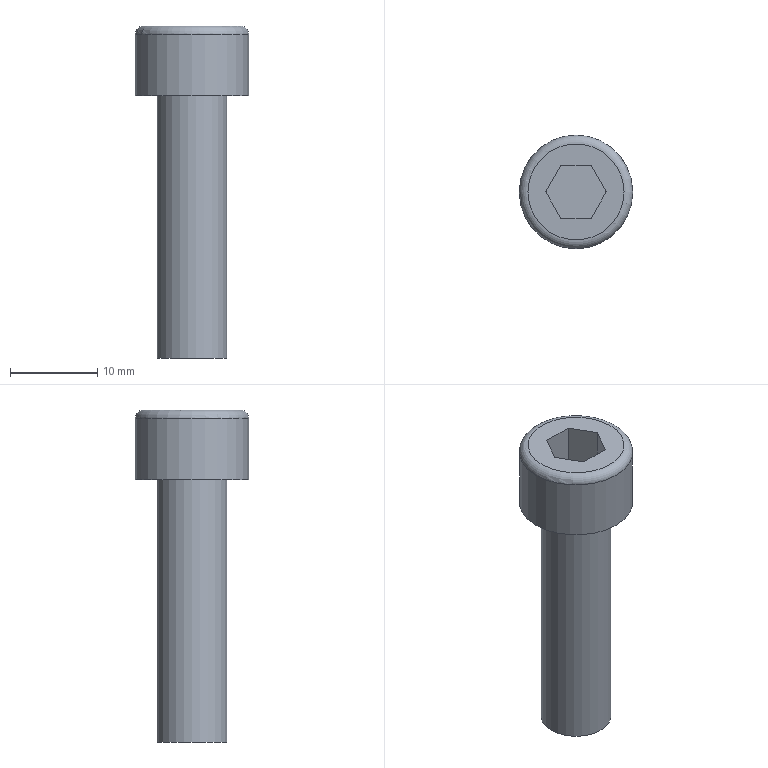Part | STEP file | Tube necking machine_id386_x_t | 1 solid | 13 faces | box 13 x 13 x 38 mm | volume 2397 mm3 | plane 10 | cylinder 2 | torus 1 | commonest cylinder face diameters 8 x1 13 x1
STEP:
#1=CARTESIAN_POINT('',(0.,0.,0.));
#2=DIRECTION('',(0.,0.,1.));
#3=DIRECTION('',(1.,0.,0.));
#4=AXIS2_PLACEMENT_3D('',#1,#2,#3);
#5=CARTESIAN_POINT('',(-164.,28.,208.));
#6=VERTEX_POINT('',#5);
#7=CARTESIAN_POINT('',(-169.5,28.,208.));
#8=DIRECTION('',(0.,0.,1.));
#9=DIRECTION('',(1.,0.,0.));
#10=AXIS2_PLACEMENT_3D('',#7,#8,#9);
#11=CIRCLE('',#10,5.5);
#12=CARTESIAN_POINT('',(-176.,28.,208.));
#13=DIRECTION('',(0.,0.,-1.));
#14=DIRECTION('',(1.,0.,0.));
#15=AXIS2_PLACEMENT_3D('',#12,#13,#14);
#16=PLANE('',#15);
#17=CARTESIAN_POINT('',(12.,0.));
#18=CARTESIAN_POINT('',(12.,-9.526));
#19=CARTESIAN_POINT('',(3.75,-4.763));
#20=CARTESIAN_POINT('',(-4.5,0.));
#21=CARTESIAN_POINT('',(3.75,4.763));
#22=CARTESIAN_POINT('',(12.,9.526));
#23=CARTESIAN_POINT('',(12.,0.));
#24=(BOUNDED_CURVE()B_SPLINE_CURVE(2,(#17,#18,#19,#20,#21,#22,#23),.UNSPECIFIED.,.T.,.F.)B_SPLINE_CURVE_WITH_KNOTS((1,2,2,2,2,1),(-2.094,0.,2.094,4.189,6.283,8.378),.UNSPECIFIED.)CURVE()GEOMETRIC_REPRESENTATION_ITEM()RATIONAL_B_SPLINE_CURVE((1.,0.5,1.,0.5,1.,0.5,1.))REPRESENTATION_ITEM(''));
#25=(GEOMETRIC_REPRESENTATION_CONTEXT(2)PARAMETRIC_REPRESENTATION_CONTEXT()REPRESENTATION_CONTEXT('',''));
#26=DEFINITIONAL_REPRESENTATION('',(#24),#25);
#27=PCURVE('',#16,#26);
#28=CARTESIAN_POINT('',(-169.5,28.,207.));
#29=DIRECTION('',(0.,0.,-1.));
#30=DIRECTION('',(1.,0.,0.));
#31=AXIS2_PLACEMENT_3D('',#28,#29,#30);
#32=TOROIDAL_SURFACE('',#31,5.5,1.);
#33=CARTESIAN_POINT('',(6.283,4.712));
#34=DIRECTION('',(-1.,0.));
#35=VECTOR('',#34,1.);
#36=LINE('',#33,#35);
#37=(GEOMETRIC_REPRESENTATION_CONTEXT(2)PARAMETRIC_REPRESENTATION_CONTEXT()REPRESENTATION_CONTEXT('',''));
#38=DEFINITIONAL_REPRESENTATION('',(#36),#37);
#39=PCURVE('',#32,#38);
#40=SURFACE_CURVE('',#11,(#27,#39),.PCURVE_S1.);
#41=EDGE_CURVE('',#6,#6,#40,.T.);
#42=ORIENTED_EDGE('',*,*,#41,.T.);
#43=EDGE_LOOP('',(#42));
#44=FACE_BOUND('',#43,.T.);
#45=CARTESIAN_POINT('',(-171.232,31.,208.));
#46=VERTEX_POINT('',#45);
#47=CARTESIAN_POINT('',(-167.768,31.,208.));
#48=VERTEX_POINT('',#47);
#49=CARTESIAN_POINT('',(-167.768,31.,208.));
#50=DIRECTION('',(1.,0.,0.));
#51=VECTOR('',#50,1.);
#52=LINE('',#49,#51);
#53=CARTESIAN_POINT('',(8.232,-3.));
#54=DIRECTION('',(1.,0.));
#55=VECTOR('',#54,1.);
#56=LINE('',#53,#55);
#57=(GEOMETRIC_REPRESENTATION_CONTEXT(2)PARAMETRIC_REPRESENTATION_CONTEXT()REPRESENTATION_CONTEXT('',''));
#58=DEFINITIONAL_REPRESENTATION('',(#56),#57);
#59=PCURVE('',#16,#58);
#60=CARTESIAN_POINT('',(-167.768,31.,202.72));
#61=DIRECTION('',(0.,-1.,0.));
#62=DIRECTION('',(-1.,0.,0.));
#63=AXIS2_PLACEMENT_3D('',#60,#61,#62);
#64=PLANE('',#63);
#65=CARTESIAN_POINT('',(0.,-5.28));
#66=DIRECTION('',(-1.,0.));
#67=VECTOR('',#66,1.);
#68=LINE('',#65,#67);
#69=(GEOMETRIC_REPRESENTATION_CONTEXT(2)PARAMETRIC_REPRESENTATION_CONTEXT()REPRESENTATION_CONTEXT('',''));
#70=DEFINITIONAL_REPRESENTATION('',(#68),#69);
#71=PCURVE('',#64,#70);
#72=SURFACE_CURVE('',#52,(#59,#71),.PCURVE_S1.);
#73=EDGE_CURVE('',#46,#48,#72,.T.);
#74=ORIENTED_EDGE('',*,*,#73,.T.);
#75=CARTESIAN_POINT('',(-166.036,28.,208.));
#76=VERTEX_POINT('',#75);
#77=CARTESIAN_POINT('',(-166.036,28.,208.));
#78=DIRECTION('',(0.5,-0.866,0.));
#79=VECTOR('',#78,1.);
#80=LINE('',#77,#79);
#81=CARTESIAN_POINT('',(9.964,0.));
#82=DIRECTION('',(0.5,0.866));
#83=VECTOR('',#82,1.);
#84=LINE('',#81,#83);
#85=(GEOMETRIC_REPRESENTATION_CONTEXT(2)PARAMETRIC_REPRESENTATION_CONTEXT()REPRESENTATION_CONTEXT('',''));
#86=DEFINITIONAL_REPRESENTATION('',(#84),#85);
#87=PCURVE('',#16,#86);
#88=CARTESIAN_POINT('',(-166.036,28.,202.72));
#89=DIRECTION('',(-0.866,-0.5,0.));
#90=DIRECTION('',(-0.5,0.866,0.));
#91=AXIS2_PLACEMENT_3D('',#88,#89,#90);
#92=PLANE('',#91);
#93=CARTESIAN_POINT('',(0.,-5.28));
#94=DIRECTION('',(-1.,0.));
#95=VECTOR('',#94,1.);
#96=LINE('',#93,#95);
#97=(GEOMETRIC_REPRESENTATION_CONTEXT(2)PARAMETRIC_REPRESENTATION_CONTEXT()REPRESENTATION_CONTEXT('',''));
#98=DEFINITIONAL_REPRESENTATION('',(#96),#97);
#99=PCURVE('',#92,#98);
#100=SURFACE_CURVE('',#80,(#87,#99),.PCURVE_S1.);
#101=EDGE_CURVE('',#48,#76,#100,.T.);
#102=ORIENTED_EDGE('',*,*,#101,.T.);
#103=CARTESIAN_POINT('',(-167.768,25.,208.));
#104=VERTEX_POINT('',#103);
#105=CARTESIAN_POINT('',(-167.768,25.,208.));
#106=DIRECTION('',(-0.5,-0.866,0.));
#107=VECTOR('',#106,1.);
#108=LINE('',#105,#107);
#109=CARTESIAN_POINT('',(8.232,3.));
#110=DIRECTION('',(-0.5,0.866));
#111=VECTOR('',#110,1.);
#112=LINE('',#109,#111);
#113=(GEOMETRIC_REPRESENTATION_CONTEXT(2)PARAMETRIC_REPRESENTATION_CONTEXT()REPRESENTATION_CONTEXT('',''));
#114=DEFINITIONAL_REPRESENTATION('',(#112),#113);
#115=PCURVE('',#16,#114);
#116=CARTESIAN_POINT('',(-167.768,25.,202.72));
#117=DIRECTION('',(-0.866,0.5,0.));
#118=DIRECTION('',(0.5,0.866,0.));
#119=AXIS2_PLACEMENT_3D('',#116,#117,#118);
#120=PLANE('',#119);
#121=CARTESIAN_POINT('',(0.,-5.28));
#122=DIRECTION('',(-1.,0.));
#123=VECTOR('',#122,1.);
#124=LINE('',#121,#123);
#125=(GEOMETRIC_REPRESENTATION_CONTEXT(2)PARAMETRIC_REPRESENTATION_CONTEXT()REPRESENTATION_CONTEXT('',''));
#126=DEFINITIONAL_REPRESENTATION('',(#124),#125);
#127=PCURVE('',#120,#126);
#128=SURFACE_CURVE('',#108,(#115,#127),.PCURVE_S1.);
#129=EDGE_CURVE('',#76,#104,#128,.T.);
#130=ORIENTED_EDGE('',*,*,#129,.T.);
#131=CARTESIAN_POINT('',(-171.232,25.,208.));
#132=VERTEX_POINT('',#131);
#133=CARTESIAN_POINT('',(-171.232,25.,208.));
#134=DIRECTION('',(-1.,0.,0.));
#135=VECTOR('',#134,1.);
#136=LINE('',#133,#135);
#137=CARTESIAN_POINT('',(4.768,3.));
#138=DIRECTION('',(-1.,0.));
#139=VECTOR('',#138,1.);
#140=LINE('',#137,#139);
#141=(GEOMETRIC_REPRESENTATION_CONTEXT(2)PARAMETRIC_REPRESENTATION_CONTEXT()REPRESENTATION_CONTEXT('',''));
#142=DEFINITIONAL_REPRESENTATION('',(#140),#141);
#143=PCURVE('',#16,#142);
#144=CARTESIAN_POINT('',(-171.232,25.,202.72));
#145=DIRECTION('',(0.,1.,0.));
#146=DIRECTION('',(1.,0.,0.));
#147=AXIS2_PLACEMENT_3D('',#144,#145,#146);
#148=PLANE('',#147);
#149=CARTESIAN_POINT('',(0.,-5.28));
#150=DIRECTION('',(-1.,0.));
#151=VECTOR('',#150,1.);
#152=LINE('',#149,#151);
#153=(GEOMETRIC_REPRESENTATION_CONTEXT(2)PARAMETRIC_REPRESENTATION_CONTEXT()REPRESENTATION_CONTEXT('',''));
#154=DEFINITIONAL_REPRESENTATION('',(#152),#153);
#155=PCURVE('',#148,#154);
#156=SURFACE_CURVE('',#136,(#143,#155),.PCURVE_S1.);
#157=EDGE_CURVE('',#104,#132,#156,.T.);
#158=ORIENTED_EDGE('',*,*,#157,.T.);
#159=CARTESIAN_POINT('',(-172.964,28.,208.));
#160=VERTEX_POINT('',#159);
#161=CARTESIAN_POINT('',(-172.964,28.,208.));
#162=DIRECTION('',(-0.5,0.866,0.));
#163=VECTOR('',#162,1.);
#164=LINE('',#161,#163);
#165=CARTESIAN_POINT('',(3.036,0.));
#166=DIRECTION('',(-0.5,-0.866));
#167=VECTOR('',#166,1.);
#168=LINE('',#165,#167);
#169=(GEOMETRIC_REPRESENTATION_CONTEXT(2)PARAMETRIC_REPRESENTATION_CONTEXT()REPRESENTATION_CONTEXT('',''));
#170=DEFINITIONAL_REPRESENTATION('',(#168),#169);
#171=PCURVE('',#16,#170);
#172=CARTESIAN_POINT('',(-172.964,28.,202.72));
#173=DIRECTION('',(0.866,0.5,0.));
#174=DIRECTION('',(0.5,-0.866,0.));
#175=AXIS2_PLACEMENT_3D('',#172,#173,#174);
#176=PLANE('',#175);
#177=CARTESIAN_POINT('',(0.,-5.28));
#178=DIRECTION('',(-1.,0.));
#179=VECTOR('',#178,1.);
#180=LINE('',#177,#179);
#181=(GEOMETRIC_REPRESENTATION_CONTEXT(2)PARAMETRIC_REPRESENTATION_CONTEXT()REPRESENTATION_CONTEXT('',''));
#182=DEFINITIONAL_REPRESENTATION('',(#180),#181);
#183=PCURVE('',#176,#182);
#184=SURFACE_CURVE('',#164,(#171,#183),.PCURVE_S1.);
#185=EDGE_CURVE('',#132,#160,#184,.T.);
#186=ORIENTED_EDGE('',*,*,#185,.T.);
#187=CARTESIAN_POINT('',(-171.232,31.,208.));
#188=DIRECTION('',(0.5,0.866,0.));
#189=VECTOR('',#188,1.);
#190=LINE('',#187,#189);
#191=CARTESIAN_POINT('',(4.768,-3.));
#192=DIRECTION('',(0.5,-0.866));
#193=VECTOR('',#192,1.);
#194=LINE('',#191,#193);
#195=(GEOMETRIC_REPRESENTATION_CONTEXT(2)PARAMETRIC_REPRESENTATION_CONTEXT()REPRESENTATION_CONTEXT('',''));
#196=DEFINITIONAL_REPRESENTATION('',(#194),#195);
#197=PCURVE('',#16,#196);
#198=CARTESIAN_POINT('',(-171.232,31.,202.72));
#199=DIRECTION('',(0.866,-0.5,0.));
#200=DIRECTION('',(-0.5,-0.866,0.));
#201=AXIS2_PLACEMENT_3D('',#198,#199,#200);
#202=PLANE('',#201);
#203=CARTESIAN_POINT('',(0.,-5.28));
#204=DIRECTION('',(-1.,0.));
#205=VECTOR('',#204,1.);
#206=LINE('',#203,#205);
#207=(GEOMETRIC_REPRESENTATION_CONTEXT(2)PARAMETRIC_REPRESENTATION_CONTEXT()REPRESENTATION_CONTEXT('',''));
#208=DEFINITIONAL_REPRESENTATION('',(#206),#207);
#209=PCURVE('',#202,#208);
#210=SURFACE_CURVE('',#190,(#197,#209),.PCURVE_S1.);
#211=EDGE_CURVE('',#160,#46,#210,.T.);
#212=ORIENTED_EDGE('',*,*,#211,.T.);
#213=EDGE_LOOP('',(#74,#102,#130,#158,#186,#212));
#214=FACE_BOUND('',#213,.T.);
#215=ADVANCED_FACE('',(#44,#214),#16,.F.);
#216=CARTESIAN_POINT('',(-163.,28.,207.));
#217=VERTEX_POINT('',#216);
#218=CARTESIAN_POINT('',(-176.,28.,207.));
#219=VERTEX_POINT('',#218);
#220=CARTESIAN_POINT('',(-169.5,28.,207.));
#221=DIRECTION('',(0.,0.,-1.));
#222=DIRECTION('',(1.,0.,0.));
#223=AXIS2_PLACEMENT_3D('',#220,#221,#222);
#224=CIRCLE('',#223,6.5);
#225=CARTESIAN_POINT('',(-169.5,28.,178.1));
#226=DIRECTION('',(0.,0.,1.));
#227=DIRECTION('',(-1.,0.,0.));
#228=AXIS2_PLACEMENT_3D('',#225,#226,#227);
#229=CYLINDRICAL_SURFACE('',#228,6.5);
#230=CARTESIAN_POINT('',(3.142,28.9));
#231=DIRECTION('',(-1.,0.));
#232=VECTOR('',#231,1.);
#233=LINE('',#230,#232);
#234=(GEOMETRIC_REPRESENTATION_CONTEXT(2)PARAMETRIC_REPRESENTATION_CONTEXT()REPRESENTATION_CONTEXT('',''));
#235=DEFINITIONAL_REPRESENTATION('',(#233),#234);
#236=PCURVE('',#229,#235);
#237=CARTESIAN_POINT('',(0.,6.283));
#238=DIRECTION('',(1.,0.));
#239=VECTOR('',#238,1.);
#240=LINE('',#237,#239);
#241=(GEOMETRIC_REPRESENTATION_CONTEXT(2)PARAMETRIC_REPRESENTATION_CONTEXT()REPRESENTATION_CONTEXT('',''));
#242=DEFINITIONAL_REPRESENTATION('',(#240),#241);
#243=PCURVE('',#32,#242);
#244=SURFACE_CURVE('',#224,(#236,#243),.PCURVE_S1.);
#245=EDGE_CURVE('',#217,#219,#244,.T.);
#246=ORIENTED_EDGE('',*,*,#245,.T.);
#247=CARTESIAN_POINT('',(-176.,28.,200.));
#248=VERTEX_POINT('',#247);
#249=CARTESIAN_POINT('',(-176.,28.,200.));
#250=CARTESIAN_POINT('',(-176.,28.,207.));
#251=B_SPLINE_CURVE_WITH_KNOTS('',1,(#249,#250),.UNSPECIFIED.,.F.,.F.,(2,2),(21.9,28.9),.PIECEWISE_BEZIER_KNOTS.);
#252=CARTESIAN_POINT('',(0.,0.));
#253=DIRECTION('',(0.,1.));
#254=VECTOR('',#253,1.);
#255=LINE('',#252,#254);
#256=(GEOMETRIC_REPRESENTATION_CONTEXT(2)PARAMETRIC_REPRESENTATION_CONTEXT()REPRESENTATION_CONTEXT('',''));
#257=DEFINITIONAL_REPRESENTATION('',(#255),#256);
#258=PCURVE('',#229,#257);
#259=CARTESIAN_POINT('',(6.283,0.));
#260=DIRECTION('',(0.,1.));
#261=VECTOR('',#260,1.);
#262=LINE('',#259,#261);
#263=(GEOMETRIC_REPRESENTATION_CONTEXT(2)PARAMETRIC_REPRESENTATION_CONTEXT()REPRESENTATION_CONTEXT('',''));
#264=DEFINITIONAL_REPRESENTATION('',(#262),#263);
#265=PCURVE('',#229,#264);
#266=SEAM_CURVE('',#251,(#258,#265),.PCURVE_S1.);
#267=EDGE_CURVE('',#248,#219,#266,.T.);
#268=ORIENTED_EDGE('',*,*,#267,.F.);
#269=CARTESIAN_POINT('',(-169.5,28.,200.));
#270=DIRECTION('',(0.,0.,1.));
#271=DIRECTION('',(-1.,0.,0.));
#272=AXIS2_PLACEMENT_3D('',#269,#270,#271);
#273=CIRCLE('',#272,6.5);
#274=CARTESIAN_POINT('',(0.,21.9));
#275=DIRECTION('',(1.,0.));
#276=VECTOR('',#275,1.);
#277=LINE('',#274,#276);
#278=(GEOMETRIC_REPRESENTATION_CONTEXT(2)PARAMETRIC_REPRESENTATION_CONTEXT()REPRESENTATION_CONTEXT('',''));
#279=DEFINITIONAL_REPRESENTATION('',(#277),#278);
#280=PCURVE('',#229,#279);
#281=CARTESIAN_POINT('',(-173.5,28.,200.));
#282=DIRECTION('',(0.,0.,1.));
#283=DIRECTION('',(-1.,0.,0.));
#284=AXIS2_PLACEMENT_3D('',#281,#282,#283);
#285=PLANE('',#284);
#286=CARTESIAN_POINT('',(-4.,0.));
#287=DIRECTION('',(1.,0.));
#288=AXIS2_PLACEMENT_2D('',#286,#287);
#289=CIRCLE('',#288,6.5);
#290=(GEOMETRIC_REPRESENTATION_CONTEXT(2)PARAMETRIC_REPRESENTATION_CONTEXT()REPRESENTATION_CONTEXT('',''));
#291=DEFINITIONAL_REPRESENTATION('',(#289),#290);
#292=PCURVE('',#285,#291);
#293=SURFACE_CURVE('',#273,(#280,#292),.PCURVE_S1.);
#294=EDGE_CURVE('',#248,#248,#293,.T.);
#295=ORIENTED_EDGE('',*,*,#294,.T.);
#296=ORIENTED_EDGE('',*,*,#267,.T.);
#297=CARTESIAN_POINT('',(-169.5,28.,207.));
#298=DIRECTION('',(0.,0.,-1.));
#299=DIRECTION('',(1.,0.,0.));
#300=AXIS2_PLACEMENT_3D('',#297,#298,#299);
#301=CIRCLE('',#300,6.5);
#302=CARTESIAN_POINT('',(9.425,28.9));
#303=DIRECTION('',(-1.,0.));
#304=VECTOR('',#303,1.);
#305=LINE('',#302,#304);
#306=(GEOMETRIC_REPRESENTATION_CONTEXT(2)PARAMETRIC_REPRESENTATION_CONTEXT()REPRESENTATION_CONTEXT('',''));
#307=DEFINITIONAL_REPRESENTATION('',(#305),#306);
#308=PCURVE('',#229,#307);
#309=CARTESIAN_POINT('',(0.,6.283));
#310=DIRECTION('',(1.,0.));
#311=VECTOR('',#310,1.);
#312=LINE('',#309,#311);
#313=(GEOMETRIC_REPRESENTATION_CONTEXT(2)PARAMETRIC_REPRESENTATION_CONTEXT()REPRESENTATION_CONTEXT('',''));
#314=DEFINITIONAL_REPRESENTATION('',(#312),#313);
#315=PCURVE('',#32,#314);
#316=SURFACE_CURVE('',#301,(#308,#315),.PCURVE_S1.);
#317=EDGE_CURVE('',#219,#217,#316,.T.);
#318=ORIENTED_EDGE('',*,*,#317,.T.);
#319=EDGE_LOOP('',(#246,#268,#295,#296,#318));
#320=FACE_BOUND('',#319,.T.);
#321=ADVANCED_FACE('',(#320),#229,.T.);
#322=ORIENTED_EDGE('',*,*,#294,.F.);
#323=EDGE_LOOP('',(#322));
#324=FACE_BOUND('',#323,.T.);
#325=CARTESIAN_POINT('',(-173.5,28.,200.));
#326=VERTEX_POINT('',#325);
#327=CARTESIAN_POINT('',(-169.5,28.,200.));
#328=DIRECTION('',(0.,0.,1.));
#329=DIRECTION('',(-1.,0.,0.));
#330=AXIS2_PLACEMENT_3D('',#327,#328,#329);
#331=CIRCLE('',#330,4.);
#332=CARTESIAN_POINT('',(-4.,0.));
#333=DIRECTION('',(1.,0.));
#334=AXIS2_PLACEMENT_2D('',#332,#333);
#335=CIRCLE('',#334,4.);
#336=(GEOMETRIC_REPRESENTATION_CONTEXT(2)PARAMETRIC_REPRESENTATION_CONTEXT()REPRESENTATION_CONTEXT('',''));
#337=DEFINITIONAL_REPRESENTATION('',(#335),#336);
#338=PCURVE('',#285,#337);
#339=CARTESIAN_POINT('',(-169.5,28.,178.1));
#340=DIRECTION('',(0.,0.,1.));
#341=DIRECTION('',(-1.,0.,0.));
#342=AXIS2_PLACEMENT_3D('',#339,#340,#341);
#343=CYLINDRICAL_SURFACE('',#342,4.);
#344=CARTESIAN_POINT('',(0.,21.9));
#345=DIRECTION('',(1.,0.));
#346=VECTOR('',#345,1.);
#347=LINE('',#344,#346);
#348=(GEOMETRIC_REPRESENTATION_CONTEXT(2)PARAMETRIC_REPRESENTATION_CONTEXT()REPRESENTATION_CONTEXT('',''));
#349=DEFINITIONAL_REPRESENTATION('',(#347),#348);
#350=PCURVE('',#343,#349);
#351=SURFACE_CURVE('',#331,(#338,#350),.PCURVE_S1.);
#352=EDGE_CURVE('',#326,#326,#351,.T.);
#353=ORIENTED_EDGE('',*,*,#352,.T.);
#354=EDGE_LOOP('',(#353));
#355=FACE_BOUND('',#354,.T.);
#356=ADVANCED_FACE('',(#324,#355),#285,.F.);
#357=ORIENTED_EDGE('',*,*,#352,.F.);
#358=CARTESIAN_POINT('',(-173.5,28.,170.));
#359=VERTEX_POINT('',#358);
#360=CARTESIAN_POINT('',(-173.5,28.,170.));
#361=CARTESIAN_POINT('',(-173.5,28.,200.));
#362=B_SPLINE_CURVE_WITH_KNOTS('',1,(#360,#361),.UNSPECIFIED.,.F.,.F.,(2,2),(-8.1,21.9),.PIECEWISE_BEZIER_KNOTS.);
#363=CARTESIAN_POINT('',(0.,0.));
#364=DIRECTION('',(0.,1.));
#365=VECTOR('',#364,1.);
#366=LINE('',#363,#365);
#367=(GEOMETRIC_REPRESENTATION_CONTEXT(2)PARAMETRIC_REPRESENTATION_CONTEXT()REPRESENTATION_CONTEXT('',''));
#368=DEFINITIONAL_REPRESENTATION('',(#366),#367);
#369=PCURVE('',#343,#368);
#370=CARTESIAN_POINT('',(6.283,0.));
#371=DIRECTION('',(0.,1.));
#372=VECTOR('',#371,1.);
#373=LINE('',#370,#372);
#374=(GEOMETRIC_REPRESENTATION_CONTEXT(2)PARAMETRIC_REPRESENTATION_CONTEXT()REPRESENTATION_CONTEXT('',''));
#375=DEFINITIONAL_REPRESENTATION('',(#373),#374);
#376=PCURVE('',#343,#375);
#377=SEAM_CURVE('',#362,(#369,#376),.PCURVE_S1.);
#378=EDGE_CURVE('',#359,#326,#377,.T.);
#379=ORIENTED_EDGE('',*,*,#378,.F.);
#380=CARTESIAN_POINT('',(-165.5,28.,170.));
#381=VERTEX_POINT('',#380);
#382=CARTESIAN_POINT('',(-169.5,28.,170.));
#383=DIRECTION('',(0.,0.,1.));
#384=DIRECTION('',(1.,0.,0.));
#385=AXIS2_PLACEMENT_3D('',#382,#383,#384);
#386=CIRCLE('',#385,4.);
#387=CARTESIAN_POINT('',(-3.142,-8.1));
#388=DIRECTION('',(1.,0.));
#389=VECTOR('',#388,1.);
#390=LINE('',#387,#389);
#391=(GEOMETRIC_REPRESENTATION_CONTEXT(2)PARAMETRIC_REPRESENTATION_CONTEXT()REPRESENTATION_CONTEXT('',''));
#392=DEFINITIONAL_REPRESENTATION('',(#390),#391);
#393=PCURVE('',#343,#392);
#394=CARTESIAN_POINT('',(-169.5,28.,170.));
#395=DIRECTION('',(0.,0.,1.));
#396=DIRECTION('',(-1.,0.,0.));
#397=AXIS2_PLACEMENT_3D('',#394,#395,#396);
#398=PLANE('',#397);
#399=CARTESIAN_POINT('',(0.,0.));
#400=DIRECTION('',(-1.,0.));
#401=AXIS2_PLACEMENT_2D('',#399,#400);
#402=CIRCLE('',#401,4.);
#403=(GEOMETRIC_REPRESENTATION_CONTEXT(2)PARAMETRIC_REPRESENTATION_CONTEXT()REPRESENTATION_CONTEXT('',''));
#404=DEFINITIONAL_REPRESENTATION('',(#402),#403);
#405=PCURVE('',#398,#404);
#406=SURFACE_CURVE('',#386,(#393,#405),.PCURVE_S1.);
#407=EDGE_CURVE('',#359,#381,#406,.T.);
#408=ORIENTED_EDGE('',*,*,#407,.T.);
#409=CARTESIAN_POINT('',(-169.5,28.,170.));
#410=DIRECTION('',(0.,0.,1.));
#411=DIRECTION('',(1.,0.,0.));
#412=AXIS2_PLACEMENT_3D('',#409,#410,#411);
#413=CIRCLE('',#412,4.);
#414=CARTESIAN_POINT('',(3.142,-8.1));
#415=DIRECTION('',(1.,0.));
#416=VECTOR('',#415,1.);
#417=LINE('',#414,#416);
#418=(GEOMETRIC_REPRESENTATION_CONTEXT(2)PARAMETRIC_REPRESENTATION_CONTEXT()REPRESENTATION_CONTEXT('',''));
#419=DEFINITIONAL_REPRESENTATION('',(#417),#418);
#420=PCURVE('',#343,#419);
#421=CARTESIAN_POINT('',(0.,0.));
#422=DIRECTION('',(-1.,0.));
#423=AXIS2_PLACEMENT_2D('',#421,#422);
#424=CIRCLE('',#423,4.);
#425=(GEOMETRIC_REPRESENTATION_CONTEXT(2)PARAMETRIC_REPRESENTATION_CONTEXT()REPRESENTATION_CONTEXT('',''));
#426=DEFINITIONAL_REPRESENTATION('',(#424),#425);
#427=PCURVE('',#398,#426);
#428=SURFACE_CURVE('',#413,(#420,#427),.PCURVE_S1.);
#429=EDGE_CURVE('',#381,#359,#428,.T.);
#430=ORIENTED_EDGE('',*,*,#429,.T.);
#431=ORIENTED_EDGE('',*,*,#378,.T.);
#432=EDGE_LOOP('',(#357,#379,#408,#430,#431));
#433=FACE_BOUND('',#432,.T.);
#434=ADVANCED_FACE('',(#433),#343,.T.);
#435=ORIENTED_EDGE('',*,*,#429,.F.);
#436=ORIENTED_EDGE('',*,*,#407,.F.);
#437=EDGE_LOOP('',(#435,#436));
#438=FACE_BOUND('',#437,.T.);
#439=ADVANCED_FACE('',(#438),#398,.F.);
#440=ORIENTED_EDGE('',*,*,#73,.F.);
#441=CARTESIAN_POINT('',(-171.232,31.,202.72));
#442=VERTEX_POINT('',#441);
#443=CARTESIAN_POINT('',(-171.232,31.,202.72));
#444=DIRECTION('',(0.,0.,1.));
#445=VECTOR('',#444,1.);
#446=LINE('',#443,#445);
#447=CARTESIAN_POINT('',(3.464,0.));
#448=DIRECTION('',(0.,-1.));
#449=VECTOR('',#448,1.);
#450=LINE('',#447,#449);
#451=(GEOMETRIC_REPRESENTATION_CONTEXT(2)PARAMETRIC_REPRESENTATION_CONTEXT()REPRESENTATION_CONTEXT('',''));
#452=DEFINITIONAL_REPRESENTATION('',(#450),#451);
#453=PCURVE('',#64,#452);
#454=CARTESIAN_POINT('',(0.,0.));
#455=DIRECTION('',(0.,-1.));
#456=VECTOR('',#455,1.);
#457=LINE('',#454,#456);
#458=(GEOMETRIC_REPRESENTATION_CONTEXT(2)PARAMETRIC_REPRESENTATION_CONTEXT()REPRESENTATION_CONTEXT('',''));
#459=DEFINITIONAL_REPRESENTATION('',(#457),#458);
#460=PCURVE('',#202,#459);
#461=SURFACE_CURVE('',#446,(#453,#460),.PCURVE_S1.);
#462=EDGE_CURVE('',#442,#46,#461,.T.);
#463=ORIENTED_EDGE('',*,*,#462,.F.);
#464=CARTESIAN_POINT('',(-167.768,31.,202.72));
#465=VERTEX_POINT('',#464);
#466=CARTESIAN_POINT('',(-167.768,31.,202.72));
#467=DIRECTION('',(-1.,0.,0.));
#468=VECTOR('',#467,1.);
#469=LINE('',#466,#468);
#470=CARTESIAN_POINT('',(0.,0.));
#471=DIRECTION('',(1.,0.));
#472=VECTOR('',#471,1.);
#473=LINE('',#470,#472);
#474=(GEOMETRIC_REPRESENTATION_CONTEXT(2)PARAMETRIC_REPRESENTATION_CONTEXT()REPRESENTATION_CONTEXT('',''));
#475=DEFINITIONAL_REPRESENTATION('',(#473),#474);
#476=PCURVE('',#64,#475);
#477=CARTESIAN_POINT('',(-169.5,28.,202.72));
#478=DIRECTION('',(0.,0.,-1.));
#479=DIRECTION('',(1.,0.,0.));
#480=AXIS2_PLACEMENT_3D('',#477,#478,#479);
#481=PLANE('',#480);
#482=CARTESIAN_POINT('',(1.732,-3.));
#483=DIRECTION('',(-1.,0.));
#484=VECTOR('',#483,1.);
#485=LINE('',#482,#484);
#486=(GEOMETRIC_REPRESENTATION_CONTEXT(2)PARAMETRIC_REPRESENTATION_CONTEXT()REPRESENTATION_CONTEXT('',''));
#487=DEFINITIONAL_REPRESENTATION('',(#485),#486);
#488=PCURVE('',#481,#487);
#489=SURFACE_CURVE('',#469,(#476,#488),.PCURVE_S1.);
#490=EDGE_CURVE('',#465,#442,#489,.T.);
#491=ORIENTED_EDGE('',*,*,#490,.F.);
#492=CARTESIAN_POINT('',(-167.768,31.,202.72));
#493=DIRECTION('',(0.,0.,1.));
#494=VECTOR('',#493,1.);
#495=LINE('',#492,#494);
#496=CARTESIAN_POINT('',(0.,0.));
#497=DIRECTION('',(0.,-1.));
#498=VECTOR('',#497,1.);
#499=LINE('',#496,#498);
#500=(GEOMETRIC_REPRESENTATION_CONTEXT(2)PARAMETRIC_REPRESENTATION_CONTEXT()REPRESENTATION_CONTEXT('',''));
#501=DEFINITIONAL_REPRESENTATION('',(#499),#500);
#502=PCURVE('',#64,#501);
#503=CARTESIAN_POINT('',(3.464,0.));
#504=DIRECTION('',(0.,-1.));
#505=VECTOR('',#504,1.);
#506=LINE('',#503,#505);
#507=(GEOMETRIC_REPRESENTATION_CONTEXT(2)PARAMETRIC_REPRESENTATION_CONTEXT()REPRESENTATION_CONTEXT('',''));
#508=DEFINITIONAL_REPRESENTATION('',(#506),#507);
#509=PCURVE('',#92,#508);
#510=SURFACE_CURVE('',#495,(#502,#509),.PCURVE_S1.);
#511=EDGE_CURVE('',#465,#48,#510,.T.);
#512=ORIENTED_EDGE('',*,*,#511,.T.);
#513=EDGE_LOOP('',(#440,#463,#491,#512));
#514=FACE_BOUND('',#513,.T.);
#515=ADVANCED_FACE('',(#514),#64,.T.);
#516=ORIENTED_EDGE('',*,*,#211,.F.);
#517=CARTESIAN_POINT('',(-172.964,28.,202.72));
#518=VERTEX_POINT('',#517);
#519=CARTESIAN_POINT('',(-172.964,28.,202.72));
#520=DIRECTION('',(0.,0.,1.));
#521=VECTOR('',#520,1.);
#522=LINE('',#519,#521);
#523=CARTESIAN_POINT('',(3.464,0.));
#524=DIRECTION('',(0.,-1.));
#525=VECTOR('',#524,1.);
#526=LINE('',#523,#525);
#527=(GEOMETRIC_REPRESENTATION_CONTEXT(2)PARAMETRIC_REPRESENTATION_CONTEXT()REPRESENTATION_CONTEXT('',''));
#528=DEFINITIONAL_REPRESENTATION('',(#526),#527);
#529=PCURVE('',#202,#528);
#530=CARTESIAN_POINT('',(0.,0.));
#531=DIRECTION('',(0.,-1.));
#532=VECTOR('',#531,1.);
#533=LINE('',#530,#532);
#534=(GEOMETRIC_REPRESENTATION_CONTEXT(2)PARAMETRIC_REPRESENTATION_CONTEXT()REPRESENTATION_CONTEXT('',''));
#535=DEFINITIONAL_REPRESENTATION('',(#533),#534);
#536=PCURVE('',#176,#535);
#537=SURFACE_CURVE('',#522,(#529,#536),.PCURVE_S1.);
#538=EDGE_CURVE('',#518,#160,#537,.T.);
#539=ORIENTED_EDGE('',*,*,#538,.F.);
#540=CARTESIAN_POINT('',(-171.232,31.,202.72));
#541=DIRECTION('',(-0.5,-0.866,0.));
#542=VECTOR('',#541,1.);
#543=LINE('',#540,#542);
#544=CARTESIAN_POINT('',(0.,0.));
#545=DIRECTION('',(1.,0.));
#546=VECTOR('',#545,1.);
#547=LINE('',#544,#546);
#548=(GEOMETRIC_REPRESENTATION_CONTEXT(2)PARAMETRIC_REPRESENTATION_CONTEXT()REPRESENTATION_CONTEXT('',''));
#549=DEFINITIONAL_REPRESENTATION('',(#547),#548);
#550=PCURVE('',#202,#549);
#551=CARTESIAN_POINT('',(-1.732,-3.));
#552=DIRECTION('',(-0.5,0.866));
#553=VECTOR('',#552,1.);
#554=LINE('',#551,#553);
#555=(GEOMETRIC_REPRESENTATION_CONTEXT(2)PARAMETRIC_REPRESENTATION_CONTEXT()REPRESENTATION_CONTEXT('',''));
#556=DEFINITIONAL_REPRESENTATION('',(#554),#555);
#557=PCURVE('',#481,#556);
#558=SURFACE_CURVE('',#543,(#550,#557),.PCURVE_S1.);
#559=EDGE_CURVE('',#442,#518,#558,.T.);
#560=ORIENTED_EDGE('',*,*,#559,.F.);
#561=ORIENTED_EDGE('',*,*,#462,.T.);
#562=EDGE_LOOP('',(#516,#539,#560,#561));
#563=FACE_BOUND('',#562,.T.);
#564=ADVANCED_FACE('',(#563),#202,.T.);
#565=ORIENTED_EDGE('',*,*,#185,.F.);
#566=CARTESIAN_POINT('',(-171.232,25.,202.72));
#567=VERTEX_POINT('',#566);
#568=CARTESIAN_POINT('',(-171.232,25.,202.72));
#569=DIRECTION('',(0.,0.,1.));
#570=VECTOR('',#569,1.);
#571=LINE('',#568,#570);
#572=CARTESIAN_POINT('',(3.464,0.));
#573=DIRECTION('',(0.,-1.));
#574=VECTOR('',#573,1.);
#575=LINE('',#572,#574);
#576=(GEOMETRIC_REPRESENTATION_CONTEXT(2)PARAMETRIC_REPRESENTATION_CONTEXT()REPRESENTATION_CONTEXT('',''));
#577=DEFINITIONAL_REPRESENTATION('',(#575),#576);
#578=PCURVE('',#176,#577);
#579=CARTESIAN_POINT('',(0.,0.));
#580=DIRECTION('',(0.,-1.));
#581=VECTOR('',#580,1.);
#582=LINE('',#579,#581);
#583=(GEOMETRIC_REPRESENTATION_CONTEXT(2)PARAMETRIC_REPRESENTATION_CONTEXT()REPRESENTATION_CONTEXT('',''));
#584=DEFINITIONAL_REPRESENTATION('',(#582),#583);
#585=PCURVE('',#148,#584);
#586=SURFACE_CURVE('',#571,(#578,#585),.PCURVE_S1.);
#587=EDGE_CURVE('',#567,#132,#586,.T.);
#588=ORIENTED_EDGE('',*,*,#587,.F.);
#589=CARTESIAN_POINT('',(-172.964,28.,202.72));
#590=DIRECTION('',(0.5,-0.866,0.));
#591=VECTOR('',#590,1.);
#592=LINE('',#589,#591);
#593=CARTESIAN_POINT('',(0.,0.));
#594=DIRECTION('',(1.,0.));
#595=VECTOR('',#594,1.);
#596=LINE('',#593,#595);
#597=(GEOMETRIC_REPRESENTATION_CONTEXT(2)PARAMETRIC_REPRESENTATION_CONTEXT()REPRESENTATION_CONTEXT('',''));
#598=DEFINITIONAL_REPRESENTATION('',(#596),#597);
#599=PCURVE('',#176,#598);
#600=CARTESIAN_POINT('',(-3.464,0.));
#601=DIRECTION('',(0.5,0.866));
#602=VECTOR('',#601,1.);
#603=LINE('',#600,#602);
#604=(GEOMETRIC_REPRESENTATION_CONTEXT(2)PARAMETRIC_REPRESENTATION_CONTEXT()REPRESENTATION_CONTEXT('',''));
#605=DEFINITIONAL_REPRESENTATION('',(#603),#604);
#606=PCURVE('',#481,#605);
#607=SURFACE_CURVE('',#592,(#599,#606),.PCURVE_S1.);
#608=EDGE_CURVE('',#518,#567,#607,.T.);
#609=ORIENTED_EDGE('',*,*,#608,.F.);
#610=ORIENTED_EDGE('',*,*,#538,.T.);
#611=EDGE_LOOP('',(#565,#588,#609,#610));
#612=FACE_BOUND('',#611,.T.);
#613=ADVANCED_FACE('',(#612),#176,.T.);
#614=ORIENTED_EDGE('',*,*,#157,.F.);
#615=CARTESIAN_POINT('',(-167.768,25.,202.72));
#616=VERTEX_POINT('',#615);
#617=CARTESIAN_POINT('',(-167.768,25.,202.72));
#618=DIRECTION('',(0.,0.,1.));
#619=VECTOR('',#618,1.);
#620=LINE('',#617,#619);
#621=CARTESIAN_POINT('',(3.464,0.));
#622=DIRECTION('',(0.,-1.));
#623=VECTOR('',#622,1.);
#624=LINE('',#621,#623);
#625=(GEOMETRIC_REPRESENTATION_CONTEXT(2)PARAMETRIC_REPRESENTATION_CONTEXT()REPRESENTATION_CONTEXT('',''));
#626=DEFINITIONAL_REPRESENTATION('',(#624),#625);
#627=PCURVE('',#148,#626);
#628=CARTESIAN_POINT('',(0.,0.));
#629=DIRECTION('',(0.,-1.));
#630=VECTOR('',#629,1.);
#631=LINE('',#628,#630);
#632=(GEOMETRIC_REPRESENTATION_CONTEXT(2)PARAMETRIC_REPRESENTATION_CONTEXT()REPRESENTATION_CONTEXT('',''));
#633=DEFINITIONAL_REPRESENTATION('',(#631),#632);
#634=PCURVE('',#120,#633);
#635=SURFACE_CURVE('',#620,(#627,#634),.PCURVE_S1.);
#636=EDGE_CURVE('',#616,#104,#635,.T.);
#637=ORIENTED_EDGE('',*,*,#636,.F.);
#638=CARTESIAN_POINT('',(-171.232,25.,202.72));
#639=DIRECTION('',(1.,0.,0.));
#640=VECTOR('',#639,1.);
#641=LINE('',#638,#640);
#642=CARTESIAN_POINT('',(0.,0.));
#643=DIRECTION('',(1.,0.));
#644=VECTOR('',#643,1.);
#645=LINE('',#642,#644);
#646=(GEOMETRIC_REPRESENTATION_CONTEXT(2)PARAMETRIC_REPRESENTATION_CONTEXT()REPRESENTATION_CONTEXT('',''));
#647=DEFINITIONAL_REPRESENTATION('',(#645),#646);
#648=PCURVE('',#148,#647);
#649=CARTESIAN_POINT('',(-1.732,3.));
#650=DIRECTION('',(1.,0.));
#651=VECTOR('',#650,1.);
#652=LINE('',#649,#651);
#653=(GEOMETRIC_REPRESENTATION_CONTEXT(2)PARAMETRIC_REPRESENTATION_CONTEXT()REPRESENTATION_CONTEXT('',''));
#654=DEFINITIONAL_REPRESENTATION('',(#652),#653);
#655=PCURVE('',#481,#654);
#656=SURFACE_CURVE('',#641,(#648,#655),.PCURVE_S1.);
#657=EDGE_CURVE('',#567,#616,#656,.T.);
#658=ORIENTED_EDGE('',*,*,#657,.F.);
#659=ORIENTED_EDGE('',*,*,#587,.T.);
#660=EDGE_LOOP('',(#614,#637,#658,#659));
#661=FACE_BOUND('',#660,.T.);
#662=ADVANCED_FACE('',(#661),#148,.T.);
#663=ORIENTED_EDGE('',*,*,#129,.F.);
#664=CARTESIAN_POINT('',(-166.036,28.,202.72));
#665=VERTEX_POINT('',#664);
#666=CARTESIAN_POINT('',(-166.036,28.,202.72));
#667=DIRECTION('',(0.,0.,1.));
#668=VECTOR('',#667,1.);
#669=LINE('',#666,#668);
#670=CARTESIAN_POINT('',(3.464,0.));
#671=DIRECTION('',(0.,-1.));
#672=VECTOR('',#671,1.);
#673=LINE('',#670,#672);
#674=(GEOMETRIC_REPRESENTATION_CONTEXT(2)PARAMETRIC_REPRESENTATION_CONTEXT()REPRESENTATION_CONTEXT('',''));
#675=DEFINITIONAL_REPRESENTATION('',(#673),#674);
#676=PCURVE('',#120,#675);
#677=CARTESIAN_POINT('',(0.,0.));
#678=DIRECTION('',(0.,-1.));
#679=VECTOR('',#678,1.);
#680=LINE('',#677,#679);
#681=(GEOMETRIC_REPRESENTATION_CONTEXT(2)PARAMETRIC_REPRESENTATION_CONTEXT()REPRESENTATION_CONTEXT('',''));
#682=DEFINITIONAL_REPRESENTATION('',(#680),#681);
#683=PCURVE('',#92,#682);
#684=SURFACE_CURVE('',#669,(#676,#683),.PCURVE_S1.);
#685=EDGE_CURVE('',#665,#76,#684,.T.);
#686=ORIENTED_EDGE('',*,*,#685,.F.);
#687=CARTESIAN_POINT('',(-167.768,25.,202.72));
#688=DIRECTION('',(0.5,0.866,0.));
#689=VECTOR('',#688,1.);
#690=LINE('',#687,#689);
#691=CARTESIAN_POINT('',(0.,0.));
#692=DIRECTION('',(1.,0.));
#693=VECTOR('',#692,1.);
#694=LINE('',#691,#693);
#695=(GEOMETRIC_REPRESENTATION_CONTEXT(2)PARAMETRIC_REPRESENTATION_CONTEXT()REPRESENTATION_CONTEXT('',''));
#696=DEFINITIONAL_REPRESENTATION('',(#694),#695);
#697=PCURVE('',#120,#696);
#698=CARTESIAN_POINT('',(1.732,3.));
#699=DIRECTION('',(0.5,-0.866));
#700=VECTOR('',#699,1.);
#701=LINE('',#698,#700);
#702=(GEOMETRIC_REPRESENTATION_CONTEXT(2)PARAMETRIC_REPRESENTATION_CONTEXT()REPRESENTATION_CONTEXT('',''));
#703=DEFINITIONAL_REPRESENTATION('',(#701),#702);
#704=PCURVE('',#481,#703);
#705=SURFACE_CURVE('',#690,(#697,#704),.PCURVE_S1.);
#706=EDGE_CURVE('',#616,#665,#705,.T.);
#707=ORIENTED_EDGE('',*,*,#706,.F.);
#708=ORIENTED_EDGE('',*,*,#636,.T.);
#709=EDGE_LOOP('',(#663,#686,#707,#708));
#710=FACE_BOUND('',#709,.T.);
#711=ADVANCED_FACE('',(#710),#120,.T.);
#712=ORIENTED_EDGE('',*,*,#101,.F.);
#713=ORIENTED_EDGE('',*,*,#511,.F.);
#714=CARTESIAN_POINT('',(-166.036,28.,202.72));
#715=DIRECTION('',(-0.5,0.866,0.));
#716=VECTOR('',#715,1.);
#717=LINE('',#714,#716);
#718=CARTESIAN_POINT('',(0.,0.));
#719=DIRECTION('',(1.,0.));
#720=VECTOR('',#719,1.);
#721=LINE('',#718,#720);
#722=(GEOMETRIC_REPRESENTATION_CONTEXT(2)PARAMETRIC_REPRESENTATION_CONTEXT()REPRESENTATION_CONTEXT('',''));
#723=DEFINITIONAL_REPRESENTATION('',(#721),#722);
#724=PCURVE('',#92,#723);
#725=CARTESIAN_POINT('',(3.464,0.));
#726=DIRECTION('',(-0.5,-0.866));
#727=VECTOR('',#726,1.);
#728=LINE('',#725,#727);
#729=(GEOMETRIC_REPRESENTATION_CONTEXT(2)PARAMETRIC_REPRESENTATION_CONTEXT()REPRESENTATION_CONTEXT('',''));
#730=DEFINITIONAL_REPRESENTATION('',(#728),#729);
#731=PCURVE('',#481,#730);
#732=SURFACE_CURVE('',#717,(#724,#731),.PCURVE_S1.);
#733=EDGE_CURVE('',#665,#465,#732,.T.);
#734=ORIENTED_EDGE('',*,*,#733,.F.);
#735=ORIENTED_EDGE('',*,*,#685,.T.);
#736=EDGE_LOOP('',(#712,#713,#734,#735));
#737=FACE_BOUND('',#736,.T.);
#738=ADVANCED_FACE('',(#737),#92,.T.);
#739=ORIENTED_EDGE('',*,*,#490,.T.);
#740=ORIENTED_EDGE('',*,*,#559,.T.);
#741=ORIENTED_EDGE('',*,*,#608,.T.);
#742=ORIENTED_EDGE('',*,*,#657,.T.);
#743=ORIENTED_EDGE('',*,*,#706,.T.);
#744=ORIENTED_EDGE('',*,*,#733,.T.);
#745=EDGE_LOOP('',(#739,#740,#741,#742,#743,#744));
#746=FACE_BOUND('',#745,.T.);
#747=ADVANCED_FACE('',(#746),#481,.F.);
#748=ORIENTED_EDGE('',*,*,#245,.F.);
#749=CARTESIAN_POINT('',(-164.,28.,208.));
#750=CARTESIAN_POINT('',(-163.733,28.,208.));
#751=CARTESIAN_POINT('',(-163.472,28.,207.915));
#752=CARTESIAN_POINT('',(-163.248,28.,207.752));
#753=CARTESIAN_POINT('',(-163.085,28.,207.528));
#754=CARTESIAN_POINT('',(-163.,28.,207.267));
#755=CARTESIAN_POINT('',(-163.,28.,207.));
#756=(BOUNDED_CURVE()B_SPLINE_CURVE(6,(#749,#750,#751,#752,#753,#754,#755),.UNSPECIFIED.,.F.,.F.)B_SPLINE_CURVE_WITH_KNOTS((7,7),(-1.571,0.),.PIECEWISE_BEZIER_KNOTS.)CURVE()GEOMETRIC_REPRESENTATION_ITEM()RATIONAL_B_SPLINE_CURVE((1.031,1.01,0.9979,0.994,0.9979,1.01,1.031))REPRESENTATION_ITEM(''));
#757=CARTESIAN_POINT('',(0.,6.283));
#758=DIRECTION('',(0.,1.));
#759=VECTOR('',#758,1.);
#760=LINE('',#757,#759);
#761=(GEOMETRIC_REPRESENTATION_CONTEXT(2)PARAMETRIC_REPRESENTATION_CONTEXT()REPRESENTATION_CONTEXT('',''));
#762=DEFINITIONAL_REPRESENTATION('',(#760),#761);
#763=PCURVE('',#32,#762);
#764=CARTESIAN_POINT('',(6.283,6.283));
#765=DIRECTION('',(0.,1.));
#766=VECTOR('',#765,1.);
#767=LINE('',#764,#766);
#768=(GEOMETRIC_REPRESENTATION_CONTEXT(2)PARAMETRIC_REPRESENTATION_CONTEXT()REPRESENTATION_CONTEXT('',''));
#769=DEFINITIONAL_REPRESENTATION('',(#767),#768);
#770=PCURVE('',#32,#769);
#771=SEAM_CURVE('',#756,(#763,#770),.PCURVE_S1.);
#772=EDGE_CURVE('',#6,#217,#771,.T.);
#773=ORIENTED_EDGE('',*,*,#772,.F.);
#774=ORIENTED_EDGE('',*,*,#41,.F.);
#775=ORIENTED_EDGE('',*,*,#772,.T.);
#776=ORIENTED_EDGE('',*,*,#317,.F.);
#777=EDGE_LOOP('',(#748,#773,#774,#775,#776));
#778=FACE_BOUND('',#777,.T.);
#779=ADVANCED_FACE('',(#778),#32,.T.);
#780=CLOSED_SHELL('',(#215,#321,#356,#434,#439,#515,#564,#613,#662,#711,#738,#747,#779));
#781=MANIFOLD_SOLID_BREP('',#780);
#782=(LENGTH_UNIT()NAMED_UNIT(*)SI_UNIT(.MILLI.,.METRE.));
#783=UNCERTAINTY_MEASURE_WITH_UNIT(LENGTH_MEASURE(0.000002),#782,'','');
#784=(NAMED_UNIT(*)PLANE_ANGLE_UNIT()SI_UNIT($,.RADIAN.));
#785=(NAMED_UNIT(*)SI_UNIT($,.STERADIAN.)SOLID_ANGLE_UNIT());
#786=(GEOMETRIC_REPRESENTATION_CONTEXT(3)GLOBAL_UNCERTAINTY_ASSIGNED_CONTEXT((#783))GLOBAL_UNIT_ASSIGNED_CONTEXT((#782,#784,#785))REPRESENTATION_CONTEXT('',''));
#787=ADVANCED_BREP_SHAPE_REPRESENTATION('',(#4,#781),#786);